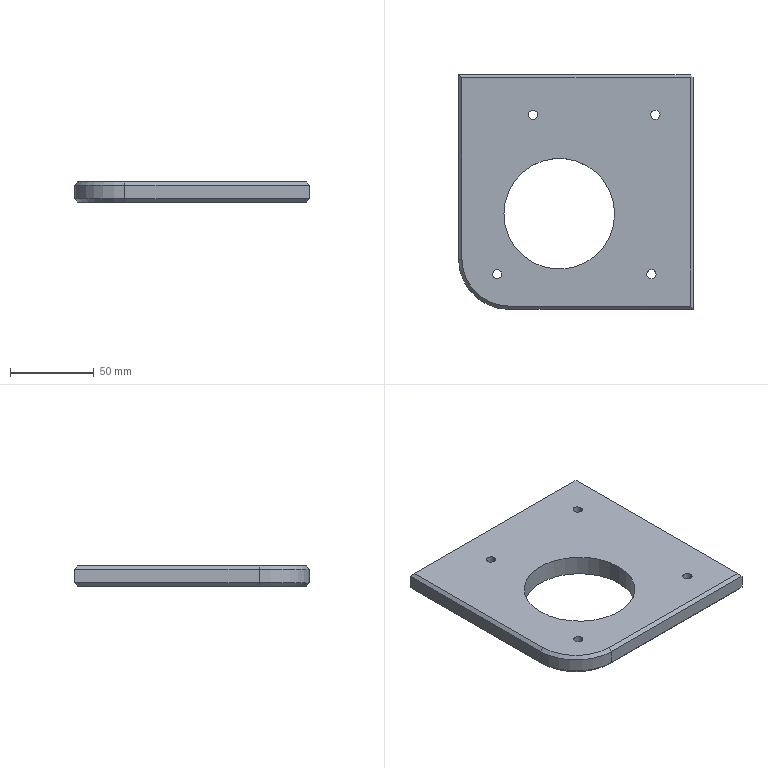Part | Creo | 1 solid | 40 faces | box 140 x 140 x 12 mm | volume 187371 mm3 | plane 19 | cylinder 19 | cone 2 | commonest cylinder face diameters 5.5 x8 9.5 x8 66 x2 60 x1
STEP:
#1=CARTESIAN_POINT('',(333.,236.995,1.));
#2=VERTEX_POINT('',#1);
#3=CARTESIAN_POINT('',(225.,236.995,1.));
#4=VERTEX_POINT('',#3);
#5=CARTESIAN_POINT('',(333.,236.995,1.));
#6=DIRECTION('',(-1.,0.,0.));
#7=VECTOR('',#6,108.);
#8=LINE('',#5,#7);
#9=EDGE_CURVE('',#2,#4,#8,.T.);
#10=ORIENTED_EDGE('',*,*,#9,.T.);
#11=CARTESIAN_POINT('',(197.,264.995,1.));
#12=VERTEX_POINT('',#11);
#13=CARTESIAN_POINT('',(225.,264.995,1.));
#14=DIRECTION('',(0.,0.,1.));
#15=DIRECTION('',(-1.,0.,0.));
#16=AXIS2_PLACEMENT_3D('',#13,#14,#15);
#17=CIRCLE('',#16,28.);
#18=EDGE_CURVE('',#12,#4,#17,.T.);
#19=ORIENTED_EDGE('',*,*,#18,.F.);
#20=CARTESIAN_POINT('',(197.,372.995,1.));
#21=VERTEX_POINT('',#20);
#22=CARTESIAN_POINT('',(197.,264.995,1.));
#23=DIRECTION('',(0.,1.,0.));
#24=VECTOR('',#23,108.);
#25=LINE('',#22,#24);
#26=EDGE_CURVE('',#12,#21,#25,.T.);
#27=ORIENTED_EDGE('',*,*,#26,.T.);
#28=CARTESIAN_POINT('',(333.,372.995,1.));
#29=VERTEX_POINT('',#28);
#30=CARTESIAN_POINT('',(197.,372.995,1.));
#31=DIRECTION('',(1.,0.,0.));
#32=VECTOR('',#31,136.);
#33=LINE('',#30,#32);
#34=EDGE_CURVE('',#21,#29,#33,.T.);
#35=ORIENTED_EDGE('',*,*,#34,.T.);
#36=CARTESIAN_POINT('',(333.,372.995,1.));
#37=DIRECTION('',(0.,-1.,0.));
#38=VECTOR('',#37,136.);
#39=LINE('',#36,#38);
#40=EDGE_CURVE('',#29,#2,#39,.T.);
#41=ORIENTED_EDGE('',*,*,#40,.T.);
#42=EDGE_LOOP('',(#10,#19,#27,#35,#41));
#43=FACE_OUTER_BOUND('',#42,.F.);
#44=CARTESIAN_POINT('',(215.25,256.,1.));
#45=VERTEX_POINT('',#44);
#46=CARTESIAN_POINT('',(220.75,256.,1.));
#47=VERTEX_POINT('',#46);
#48=CARTESIAN_POINT('',(218.,256.,1.));
#49=DIRECTION('',(0.,0.,-1.));
#50=DIRECTION('',(-1.,0.,0.));
#51=AXIS2_PLACEMENT_3D('',#48,#49,#50);
#52=CIRCLE('',#51,2.75);
#53=EDGE_CURVE('',#45,#47,#52,.T.);
#54=ORIENTED_EDGE('',*,*,#53,.F.);
#55=CARTESIAN_POINT('',(218.,256.,1.));
#56=DIRECTION('',(0.,0.,-1.));
#57=DIRECTION('',(1.,0.,0.));
#58=AXIS2_PLACEMENT_3D('',#55,#56,#57);
#59=CIRCLE('',#58,2.75);
#60=EDGE_CURVE('',#47,#45,#59,.T.);
#61=ORIENTED_EDGE('',*,*,#60,.F.);
#62=EDGE_LOOP('',(#54,#61));
#63=FACE_BOUND('',#62,.F.);
#64=CARTESIAN_POINT('',(236.618,351.,1.));
#65=VERTEX_POINT('',#64);
#66=CARTESIAN_POINT('',(242.118,351.,1.));
#67=VERTEX_POINT('',#66);
#68=CARTESIAN_POINT('',(239.368,351.,1.));
#69=DIRECTION('',(0.,0.,-1.));
#70=DIRECTION('',(-1.,0.,0.));
#71=AXIS2_PLACEMENT_3D('',#68,#69,#70);
#72=CIRCLE('',#71,2.75);
#73=EDGE_CURVE('',#65,#67,#72,.T.);
#74=ORIENTED_EDGE('',*,*,#73,.F.);
#75=CARTESIAN_POINT('',(239.368,351.,1.));
#76=DIRECTION('',(0.,0.,-1.));
#77=DIRECTION('',(1.,0.,0.));
#78=AXIS2_PLACEMENT_3D('',#75,#76,#77);
#79=CIRCLE('',#78,2.75);
#80=EDGE_CURVE('',#67,#65,#79,.T.);
#81=ORIENTED_EDGE('',*,*,#80,.F.);
#82=EDGE_LOOP('',(#74,#81));
#83=FACE_BOUND('',#82,.F.);
#84=CARTESIAN_POINT('',(288.,291.995,1.));
#85=VERTEX_POINT('',#84);
#86=CARTESIAN_POINT('',(222.,291.995,1.));
#87=VERTEX_POINT('',#86);
#88=CARTESIAN_POINT('',(255.,291.995,1.));
#89=DIRECTION('',(0.,0.,-1.));
#90=DIRECTION('',(1.,0.,0.));
#91=AXIS2_PLACEMENT_3D('',#88,#89,#90);
#92=CIRCLE('',#91,33.);
#93=EDGE_CURVE('',#85,#87,#92,.T.);
#94=ORIENTED_EDGE('',*,*,#93,.F.);
#95=CARTESIAN_POINT('',(255.,291.995,1.));
#96=DIRECTION('',(0.,0.,-1.));
#97=DIRECTION('',(-1.,0.,0.));
#98=AXIS2_PLACEMENT_3D('',#95,#96,#97);
#99=CIRCLE('',#98,33.);
#100=EDGE_CURVE('',#87,#85,#99,.T.);
#101=ORIENTED_EDGE('',*,*,#100,.F.);
#102=EDGE_LOOP('',(#94,#101));
#103=FACE_BOUND('',#102,.F.);
#104=CARTESIAN_POINT('',(309.618,351.,1.));
#105=VERTEX_POINT('',#104);
#106=CARTESIAN_POINT('',(315.118,351.,1.));
#107=VERTEX_POINT('',#106);
#108=CARTESIAN_POINT('',(312.368,351.,1.));
#109=DIRECTION('',(0.,0.,-1.));
#110=DIRECTION('',(-1.,0.,0.));
#111=AXIS2_PLACEMENT_3D('',#108,#109,#110);
#112=CIRCLE('',#111,2.75);
#113=EDGE_CURVE('',#105,#107,#112,.T.);
#114=ORIENTED_EDGE('',*,*,#113,.F.);
#115=CARTESIAN_POINT('',(312.368,351.,1.));
#116=DIRECTION('',(0.,0.,-1.));
#117=DIRECTION('',(1.,0.,0.));
#118=AXIS2_PLACEMENT_3D('',#115,#116,#117);
#119=CIRCLE('',#118,2.75);
#120=EDGE_CURVE('',#107,#105,#119,.T.);
#121=ORIENTED_EDGE('',*,*,#120,.F.);
#122=EDGE_LOOP('',(#114,#121));
#123=FACE_BOUND('',#122,.F.);
#124=CARTESIAN_POINT('',(307.25,256.,1.));
#125=VERTEX_POINT('',#124);
#126=CARTESIAN_POINT('',(312.75,256.,1.));
#127=VERTEX_POINT('',#126);
#128=CARTESIAN_POINT('',(310.,256.,1.));
#129=DIRECTION('',(0.,0.,-1.));
#130=DIRECTION('',(-1.,0.,0.));
#131=AXIS2_PLACEMENT_3D('',#128,#129,#130);
#132=CIRCLE('',#131,2.75);
#133=EDGE_CURVE('',#125,#127,#132,.T.);
#134=ORIENTED_EDGE('',*,*,#133,.F.);
#135=CARTESIAN_POINT('',(310.,256.,1.));
#136=DIRECTION('',(0.,0.,-1.));
#137=DIRECTION('',(1.,0.,0.));
#138=AXIS2_PLACEMENT_3D('',#135,#136,#137);
#139=CIRCLE('',#138,2.75);
#140=EDGE_CURVE('',#127,#125,#139,.T.);
#141=ORIENTED_EDGE('',*,*,#140,.F.);
#142=EDGE_LOOP('',(#134,#141));
#143=FACE_BOUND('',#142,.F.);
#144=CARTESIAN_POINT('',(265.,302.495,1.));
#145=DIRECTION('',(0.,0.,1.));
#146=DIRECTION('',(-1.,0.,0.));
#147=AXIS2_PLACEMENT_3D('',#144,#145,#146);
#148=PLANE('',#147);
#149=ADVANCED_FACE('',(#43,#63,#83,#103,#123,#143),#148,.T.);
#150=CARTESIAN_POINT('',(225.,234.995,-1.));
#151=VERTEX_POINT('',#150);
#152=CARTESIAN_POINT('',(335.,234.995,-1.));
#153=VERTEX_POINT('',#152);
#154=CARTESIAN_POINT('',(225.,234.995,-1.));
#155=DIRECTION('',(1.,0.,0.));
#156=VECTOR('',#155,110.);
#157=LINE('',#154,#156);
#158=EDGE_CURVE('',#151,#153,#157,.T.);
#159=ORIENTED_EDGE('',*,*,#158,.F.);
#160=CARTESIAN_POINT('',(225.,234.995,-1.));
#161=DIRECTION('',(0.,0.7071,0.7071));
#162=VECTOR('',#161,2.828);
#163=LINE('',#160,#162);
#164=EDGE_CURVE('',#151,#4,#163,.T.);
#165=ORIENTED_EDGE('',*,*,#164,.T.);
#166=ORIENTED_EDGE('',*,*,#9,.F.);
#167=CARTESIAN_POINT('',(333.,236.995,1.));
#168=DIRECTION('',(0.5774,-0.5774,-0.5774));
#169=VECTOR('',#168,3.464);
#170=LINE('',#167,#169);
#171=EDGE_CURVE('',#2,#153,#170,.T.);
#172=ORIENTED_EDGE('',*,*,#171,.T.);
#173=EDGE_LOOP('',(#159,#165,#166,#172));
#174=FACE_OUTER_BOUND('',#173,.F.);
#175=CARTESIAN_POINT('',(265.,234.995,-1.));
#176=DIRECTION('',(0.,0.7071,-0.7071));
#177=DIRECTION('',(-1.,0.,0.));
#178=AXIS2_PLACEMENT_3D('',#175,#176,#177);
#179=PLANE('',#178);
#180=ADVANCED_FACE('',(#174),#179,.F.);
#181=CARTESIAN_POINT('',(225.,234.995,-9.));
#182=VERTEX_POINT('',#181);
#183=CARTESIAN_POINT('',(225.,234.995,-9.));
#184=DIRECTION('',(0.,0.,1.));
#185=VECTOR('',#184,8.);
#186=LINE('',#183,#185);
#187=EDGE_CURVE('',#182,#151,#186,.T.);
#188=ORIENTED_EDGE('',*,*,#187,.T.);
#189=ORIENTED_EDGE('',*,*,#158,.T.);
#190=CARTESIAN_POINT('',(335.,234.995,-9.));
#191=VERTEX_POINT('',#190);
#192=CARTESIAN_POINT('',(335.,234.995,-1.));
#193=DIRECTION('',(0.,0.,-1.));
#194=VECTOR('',#193,8.);
#195=LINE('',#192,#194);
#196=EDGE_CURVE('',#153,#191,#195,.T.);
#197=ORIENTED_EDGE('',*,*,#196,.T.);
#198=CARTESIAN_POINT('',(335.,234.995,-9.));
#199=DIRECTION('',(-1.,0.,0.));
#200=VECTOR('',#199,110.);
#201=LINE('',#198,#200);
#202=EDGE_CURVE('',#191,#182,#201,.T.);
#203=ORIENTED_EDGE('',*,*,#202,.T.);
#204=EDGE_LOOP('',(#188,#189,#197,#203));
#205=FACE_OUTER_BOUND('',#204,.F.);
#206=CARTESIAN_POINT('',(265.,234.995,-11.));
#207=DIRECTION('',(0.,-1.,0.));
#208=DIRECTION('',(0.,0.,1.));
#209=AXIS2_PLACEMENT_3D('',#206,#207,#208);
#210=PLANE('',#209);
#211=ADVANCED_FACE('',(#205),#210,.T.);
#212=CARTESIAN_POINT('',(195.,264.995,-1.));
#213=VERTEX_POINT('',#212);
#214=CARTESIAN_POINT('',(195.,264.995,-9.));
#215=VERTEX_POINT('',#214);
#216=CARTESIAN_POINT('',(195.,264.995,-1.));
#217=DIRECTION('',(0.,0.,-1.));
#218=VECTOR('',#217,8.);
#219=LINE('',#216,#218);
#220=EDGE_CURVE('',#213,#215,#219,.T.);
#221=ORIENTED_EDGE('',*,*,#220,.F.);
#222=CARTESIAN_POINT('',(225.,264.995,-1.));
#223=DIRECTION('',(0.,0.,1.));
#224=DIRECTION('',(-1.,0.,0.));
#225=AXIS2_PLACEMENT_3D('',#222,#223,#224);
#226=CIRCLE('',#225,30.);
#227=EDGE_CURVE('',#213,#151,#226,.T.);
#228=ORIENTED_EDGE('',*,*,#227,.T.);
#229=ORIENTED_EDGE('',*,*,#187,.F.);
#230=CARTESIAN_POINT('',(225.,264.995,-9.));
#231=DIRECTION('',(0.,0.,-1.));
#232=DIRECTION('',(0.,-1.,0.));
#233=AXIS2_PLACEMENT_3D('',#230,#231,#232);
#234=CIRCLE('',#233,30.);
#235=EDGE_CURVE('',#182,#215,#234,.T.);
#236=ORIENTED_EDGE('',*,*,#235,.T.);
#237=EDGE_LOOP('',(#221,#228,#229,#236));
#238=FACE_OUTER_BOUND('',#237,.F.);
#239=CARTESIAN_POINT('',(225.,264.995,-11.));
#240=DIRECTION('',(0.,0.,1.));
#241=DIRECTION('',(-1.,0.,0.));
#242=AXIS2_PLACEMENT_3D('',#239,#240,#241);
#243=CYLINDRICAL_SURFACE('',#242,30.);
#244=ADVANCED_FACE('',(#238),#243,.T.);
#245=CARTESIAN_POINT('',(195.,374.995,-1.));
#246=VERTEX_POINT('',#245);
#247=CARTESIAN_POINT('',(195.,374.995,-9.));
#248=VERTEX_POINT('',#247);
#249=CARTESIAN_POINT('',(195.,374.995,-1.));
#250=DIRECTION('',(0.,0.,-1.));
#251=VECTOR('',#250,8.);
#252=LINE('',#249,#251);
#253=EDGE_CURVE('',#246,#248,#252,.T.);
#254=ORIENTED_EDGE('',*,*,#253,.F.);
#255=CARTESIAN_POINT('',(195.,374.995,-1.));
#256=DIRECTION('',(0.,-1.,0.));
#257=VECTOR('',#256,110.);
#258=LINE('',#255,#257);
#259=EDGE_CURVE('',#246,#213,#258,.T.);
#260=ORIENTED_EDGE('',*,*,#259,.T.);
#261=ORIENTED_EDGE('',*,*,#220,.T.);
#262=CARTESIAN_POINT('',(195.,264.995,-9.));
#263=DIRECTION('',(0.,1.,0.));
#264=VECTOR('',#263,110.);
#265=LINE('',#262,#264);
#266=EDGE_CURVE('',#215,#248,#265,.T.);
#267=ORIENTED_EDGE('',*,*,#266,.T.);
#268=EDGE_LOOP('',(#254,#260,#261,#267));
#269=FACE_OUTER_BOUND('',#268,.F.);
#270=CARTESIAN_POINT('',(195.,302.495,-11.));
#271=DIRECTION('',(-1.,0.,0.));
#272=DIRECTION('',(0.,0.,-1.));
#273=AXIS2_PLACEMENT_3D('',#270,#271,#272);
#274=PLANE('',#273);
#275=ADVANCED_FACE('',(#269),#274,.T.);
#276=ORIENTED_EDGE('',*,*,#253,.T.);
#277=CARTESIAN_POINT('',(333.,374.995,-9.));
#278=VERTEX_POINT('',#277);
#279=CARTESIAN_POINT('',(195.,374.995,-9.));
#280=DIRECTION('',(1.,0.,0.));
#281=VECTOR('',#280,138.);
#282=LINE('',#279,#281);
#283=EDGE_CURVE('',#248,#278,#282,.T.);
#284=ORIENTED_EDGE('',*,*,#283,.T.);
#285=CARTESIAN_POINT('',(333.,374.995,-1.));
#286=VERTEX_POINT('',#285);
#287=CARTESIAN_POINT('',(333.,374.995,-9.));
#288=DIRECTION('',(0.,0.,1.));
#289=VECTOR('',#288,8.);
#290=LINE('',#287,#289);
#291=EDGE_CURVE('',#278,#286,#290,.T.);
#292=ORIENTED_EDGE('',*,*,#291,.T.);
#293=CARTESIAN_POINT('',(333.,374.995,-1.));
#294=DIRECTION('',(-1.,0.,0.));
#295=VECTOR('',#294,138.);
#296=LINE('',#293,#295);
#297=EDGE_CURVE('',#286,#246,#296,.T.);
#298=ORIENTED_EDGE('',*,*,#297,.T.);
#299=EDGE_LOOP('',(#276,#284,#292,#298));
#300=FACE_OUTER_BOUND('',#299,.F.);
#301=CARTESIAN_POINT('',(285.,374.995,165.));
#302=DIRECTION('',(0.,1.,0.));
#303=DIRECTION('',(0.,0.,-1.));
#304=AXIS2_PLACEMENT_3D('',#301,#302,#303);
#305=PLANE('',#304);
#306=ADVANCED_FACE('',(#300),#305,.T.);
#307=CARTESIAN_POINT('',(333.,372.995,-11.));
#308=VERTEX_POINT('',#307);
#309=CARTESIAN_POINT('',(197.,372.995,-11.));
#310=VERTEX_POINT('',#309);
#311=CARTESIAN_POINT('',(333.,372.995,-11.));
#312=DIRECTION('',(-1.,0.,0.));
#313=VECTOR('',#312,136.);
#314=LINE('',#311,#313);
#315=EDGE_CURVE('',#308,#310,#314,.T.);
#316=ORIENTED_EDGE('',*,*,#315,.F.);
#317=CARTESIAN_POINT('',(334.,373.995,-10.));
#318=VERTEX_POINT('',#317);
#319=CARTESIAN_POINT('',(333.,372.995,-11.));
#320=DIRECTION('',(0.5774,0.5774,0.5774));
#321=VECTOR('',#320,1.732);
#322=LINE('',#319,#321);
#323=EDGE_CURVE('',#308,#318,#322,.T.);
#324=ORIENTED_EDGE('',*,*,#323,.T.);
#325=CARTESIAN_POINT('',(334.,373.995,-10.));
#326=DIRECTION('',(-0.5774,0.5774,0.5774));
#327=VECTOR('',#326,1.732);
#328=LINE('',#325,#327);
#329=EDGE_CURVE('',#318,#278,#328,.T.);
#330=ORIENTED_EDGE('',*,*,#329,.T.);
#331=ORIENTED_EDGE('',*,*,#283,.F.);
#332=CARTESIAN_POINT('',(195.,374.995,-9.));
#333=DIRECTION('',(0.5774,-0.5774,-0.5774));
#334=VECTOR('',#333,3.464);
#335=LINE('',#332,#334);
#336=EDGE_CURVE('',#248,#310,#335,.T.);
#337=ORIENTED_EDGE('',*,*,#336,.T.);
#338=EDGE_LOOP('',(#316,#324,#330,#331,#337));
#339=FACE_OUTER_BOUND('',#338,.F.);
#340=CARTESIAN_POINT('',(285.,374.995,-9.));
#341=DIRECTION('',(0.,-0.7071,0.7071));
#342=DIRECTION('',(-1.,0.,0.));
#343=AXIS2_PLACEMENT_3D('',#340,#341,#342);
#344=PLANE('',#343);
#345=ADVANCED_FACE('',(#339),#344,.F.);
#346=CARTESIAN_POINT('',(225.,236.995,-11.));
#347=VERTEX_POINT('',#346);
#348=CARTESIAN_POINT('',(197.,264.995,-11.));
#349=VERTEX_POINT('',#348);
#350=CARTESIAN_POINT('',(225.,264.995,-11.));
#351=DIRECTION('',(0.,0.,-1.));
#352=DIRECTION('',(0.,-1.,0.));
#353=AXIS2_PLACEMENT_3D('',#350,#351,#352);
#354=CIRCLE('',#353,28.);
#355=EDGE_CURVE('',#347,#349,#354,.T.);
#356=ORIENTED_EDGE('',*,*,#355,.F.);
#357=CARTESIAN_POINT('',(333.,236.995,-11.));
#358=VERTEX_POINT('',#357);
#359=CARTESIAN_POINT('',(225.,236.995,-11.));
#360=DIRECTION('',(1.,0.,0.));
#361=VECTOR('',#360,108.);
#362=LINE('',#359,#361);
#363=EDGE_CURVE('',#347,#358,#362,.T.);
#364=ORIENTED_EDGE('',*,*,#363,.T.);
#365=CARTESIAN_POINT('',(333.,236.995,-11.));
#366=DIRECTION('',(0.,1.,0.));
#367=VECTOR('',#366,136.);
#368=LINE('',#365,#367);
#369=EDGE_CURVE('',#358,#308,#368,.T.);
#370=ORIENTED_EDGE('',*,*,#369,.T.);
#371=ORIENTED_EDGE('',*,*,#315,.T.);
#372=CARTESIAN_POINT('',(197.,372.995,-11.));
#373=DIRECTION('',(0.,-1.,0.));
#374=VECTOR('',#373,108.);
#375=LINE('',#372,#374);
#376=EDGE_CURVE('',#310,#349,#375,.T.);
#377=ORIENTED_EDGE('',*,*,#376,.T.);
#378=EDGE_LOOP('',(#356,#364,#370,#371,#377));
#379=FACE_OUTER_BOUND('',#378,.F.);
#380=CARTESIAN_POINT('',(213.25,256.,-11.));
#381=VERTEX_POINT('',#380);
#382=CARTESIAN_POINT('',(222.75,256.,-11.));
#383=VERTEX_POINT('',#382);
#384=CARTESIAN_POINT('',(218.,256.,-11.));
#385=DIRECTION('',(0.,0.,1.));
#386=DIRECTION('',(-1.,0.,0.));
#387=AXIS2_PLACEMENT_3D('',#384,#385,#386);
#388=CIRCLE('',#387,4.75);
#389=EDGE_CURVE('',#381,#383,#388,.T.);
#390=ORIENTED_EDGE('',*,*,#389,.F.);
#391=CARTESIAN_POINT('',(218.,256.,-11.));
#392=DIRECTION('',(0.,0.,1.));
#393=DIRECTION('',(1.,0.,0.));
#394=AXIS2_PLACEMENT_3D('',#391,#392,#393);
#395=CIRCLE('',#394,4.75);
#396=EDGE_CURVE('',#383,#381,#395,.T.);
#397=ORIENTED_EDGE('',*,*,#396,.F.);
#398=EDGE_LOOP('',(#390,#397));
#399=FACE_BOUND('',#398,.F.);
#400=CARTESIAN_POINT('',(307.618,351.,-11.));
#401=VERTEX_POINT('',#400);
#402=CARTESIAN_POINT('',(317.118,351.,-11.));
#403=VERTEX_POINT('',#402);
#404=CARTESIAN_POINT('',(312.368,351.,-11.));
#405=DIRECTION('',(0.,0.,1.));
#406=DIRECTION('',(-1.,0.,0.));
#407=AXIS2_PLACEMENT_3D('',#404,#405,#406);
#408=CIRCLE('',#407,4.75);
#409=EDGE_CURVE('',#401,#403,#408,.T.);
#410=ORIENTED_EDGE('',*,*,#409,.F.);
#411=CARTESIAN_POINT('',(312.368,351.,-11.));
#412=DIRECTION('',(0.,0.,1.));
#413=DIRECTION('',(1.,0.,0.));
#414=AXIS2_PLACEMENT_3D('',#411,#412,#413);
#415=CIRCLE('',#414,4.75);
#416=EDGE_CURVE('',#403,#401,#415,.T.);
#417=ORIENTED_EDGE('',*,*,#416,.F.);
#418=EDGE_LOOP('',(#410,#417));
#419=FACE_BOUND('',#418,.F.);
#420=CARTESIAN_POINT('',(234.618,351.,-11.));
#421=VERTEX_POINT('',#420);
#422=CARTESIAN_POINT('',(244.118,351.,-11.));
#423=VERTEX_POINT('',#422);
#424=CARTESIAN_POINT('',(239.368,351.,-11.));
#425=DIRECTION('',(0.,0.,1.));
#426=DIRECTION('',(-1.,0.,0.));
#427=AXIS2_PLACEMENT_3D('',#424,#425,#426);
#428=CIRCLE('',#427,4.75);
#429=EDGE_CURVE('',#421,#423,#428,.T.);
#430=ORIENTED_EDGE('',*,*,#429,.F.);
#431=CARTESIAN_POINT('',(239.368,351.,-11.));
#432=DIRECTION('',(0.,0.,1.));
#433=DIRECTION('',(1.,0.,0.));
#434=AXIS2_PLACEMENT_3D('',#431,#432,#433);
#435=CIRCLE('',#434,4.75);
#436=EDGE_CURVE('',#423,#421,#435,.T.);
#437=ORIENTED_EDGE('',*,*,#436,.F.);
#438=EDGE_LOOP('',(#430,#437));
#439=FACE_BOUND('',#438,.F.);
#440=CARTESIAN_POINT('',(305.25,256.,-11.));
#441=VERTEX_POINT('',#440);
#442=CARTESIAN_POINT('',(314.75,256.,-11.));
#443=VERTEX_POINT('',#442);
#444=CARTESIAN_POINT('',(310.,256.,-11.));
#445=DIRECTION('',(0.,0.,1.));
#446=DIRECTION('',(-1.,0.,0.));
#447=AXIS2_PLACEMENT_3D('',#444,#445,#446);
#448=CIRCLE('',#447,4.75);
#449=EDGE_CURVE('',#441,#443,#448,.T.);
#450=ORIENTED_EDGE('',*,*,#449,.F.);
#451=CARTESIAN_POINT('',(310.,256.,-11.));
#452=DIRECTION('',(0.,0.,1.));
#453=DIRECTION('',(1.,0.,0.));
#454=AXIS2_PLACEMENT_3D('',#451,#452,#453);
#455=CIRCLE('',#454,4.75);
#456=EDGE_CURVE('',#443,#441,#455,.T.);
#457=ORIENTED_EDGE('',*,*,#456,.F.);
#458=EDGE_LOOP('',(#450,#457));
#459=FACE_BOUND('',#458,.F.);
#460=CARTESIAN_POINT('',(222.,291.995,-11.));
#461=VERTEX_POINT('',#460);
#462=CARTESIAN_POINT('',(288.,291.995,-11.));
#463=VERTEX_POINT('',#462);
#464=CARTESIAN_POINT('',(255.,291.995,-11.));
#465=DIRECTION('',(0.,0.,1.));
#466=DIRECTION('',(-1.,0.,0.));
#467=AXIS2_PLACEMENT_3D('',#464,#465,#466);
#468=CIRCLE('',#467,33.);
#469=EDGE_CURVE('',#461,#463,#468,.T.);
#470=ORIENTED_EDGE('',*,*,#469,.F.);
#471=CARTESIAN_POINT('',(255.,291.995,-11.));
#472=DIRECTION('',(0.,0.,1.));
#473=DIRECTION('',(1.,0.,0.));
#474=AXIS2_PLACEMENT_3D('',#471,#472,#473);
#475=CIRCLE('',#474,33.);
#476=EDGE_CURVE('',#463,#461,#475,.T.);
#477=ORIENTED_EDGE('',*,*,#476,.F.);
#478=EDGE_LOOP('',(#470,#477));
#479=FACE_BOUND('',#478,.F.);
#480=CARTESIAN_POINT('',(265.,302.495,-11.));
#481=DIRECTION('',(0.,0.,-1.));
#482=DIRECTION('',(1.,0.,0.));
#483=AXIS2_PLACEMENT_3D('',#480,#481,#482);
#484=PLANE('',#483);
#485=ADVANCED_FACE('',(#379,#399,#419,#439,#459,#479),#484,.T.);
#486=CARTESIAN_POINT('',(314.75,256.,-5.));
#487=VERTEX_POINT('',#486);
#488=CARTESIAN_POINT('',(305.25,256.,-5.));
#489=VERTEX_POINT('',#488);
#490=CARTESIAN_POINT('',(310.,256.,-5.));
#491=DIRECTION('',(0.,0.,-1.));
#492=DIRECTION('',(1.,0.,0.));
#493=AXIS2_PLACEMENT_3D('',#490,#491,#492);
#494=CIRCLE('',#493,4.75);
#495=EDGE_CURVE('',#487,#489,#494,.T.);
#496=ORIENTED_EDGE('',*,*,#495,.T.);
#497=CARTESIAN_POINT('',(305.25,256.,-5.));
#498=DIRECTION('',(0.,0.,-1.));
#499=VECTOR('',#498,6.);
#500=LINE('',#497,#499);
#501=EDGE_CURVE('',#489,#441,#500,.T.);
#502=ORIENTED_EDGE('',*,*,#501,.T.);
#503=ORIENTED_EDGE('',*,*,#449,.T.);
#504=CARTESIAN_POINT('',(314.75,256.,-5.));
#505=DIRECTION('',(0.,0.,-1.));
#506=VECTOR('',#505,6.);
#507=LINE('',#504,#506);
#508=EDGE_CURVE('',#487,#443,#507,.T.);
#509=ORIENTED_EDGE('',*,*,#508,.F.);
#510=EDGE_LOOP('',(#496,#502,#503,#509));
#511=FACE_OUTER_BOUND('',#510,.F.);
#512=CARTESIAN_POINT('',(310.,256.,-11.));
#513=DIRECTION('',(0.,0.,-1.));
#514=DIRECTION('',(-1.,0.,0.));
#515=AXIS2_PLACEMENT_3D('',#512,#513,#514);
#516=CYLINDRICAL_SURFACE('',#515,4.75);
#517=ADVANCED_FACE('',(#511),#516,.F.);
#518=CARTESIAN_POINT('',(310.,256.,-5.));
#519=DIRECTION('',(0.,0.,-1.));
#520=DIRECTION('',(-1.,0.,0.));
#521=AXIS2_PLACEMENT_3D('',#518,#519,#520);
#522=CIRCLE('',#521,4.75);
#523=EDGE_CURVE('',#489,#487,#522,.T.);
#524=ORIENTED_EDGE('',*,*,#523,.F.);
#525=ORIENTED_EDGE('',*,*,#495,.F.);
#526=EDGE_LOOP('',(#524,#525));
#527=FACE_OUTER_BOUND('',#526,.F.);
#528=CARTESIAN_POINT('',(307.25,256.,-5.));
#529=VERTEX_POINT('',#528);
#530=CARTESIAN_POINT('',(312.75,256.,-5.));
#531=VERTEX_POINT('',#530);
#532=CARTESIAN_POINT('',(310.,256.,-5.));
#533=DIRECTION('',(0.,0.,1.));
#534=DIRECTION('',(-1.,0.,0.));
#535=AXIS2_PLACEMENT_3D('',#532,#533,#534);
#536=CIRCLE('',#535,2.75);
#537=EDGE_CURVE('',#529,#531,#536,.T.);
#538=ORIENTED_EDGE('',*,*,#537,.F.);
#539=CARTESIAN_POINT('',(310.,256.,-5.));
#540=DIRECTION('',(0.,0.,1.));
#541=DIRECTION('',(1.,0.,0.));
#542=AXIS2_PLACEMENT_3D('',#539,#540,#541);
#543=CIRCLE('',#542,2.75);
#544=EDGE_CURVE('',#531,#529,#543,.T.);
#545=ORIENTED_EDGE('',*,*,#544,.F.);
#546=EDGE_LOOP('',(#538,#545));
#547=FACE_BOUND('',#546,.F.);
#548=CARTESIAN_POINT('',(310.,260.75,-5.));
#549=DIRECTION('',(0.,0.,1.));
#550=DIRECTION('',(1.,0.,0.));
#551=AXIS2_PLACEMENT_3D('',#548,#549,#550);
#552=PLANE('',#551);
#553=ADVANCED_FACE('',(#527,#547),#552,.F.);
#554=ORIENTED_EDGE('',*,*,#140,.T.);
#555=CARTESIAN_POINT('',(307.25,256.,1.));
#556=DIRECTION('',(0.,0.,-1.));
#557=VECTOR('',#556,6.);
#558=LINE('',#555,#557);
#559=EDGE_CURVE('',#125,#529,#558,.T.);
#560=ORIENTED_EDGE('',*,*,#559,.T.);
#561=ORIENTED_EDGE('',*,*,#537,.T.);
#562=CARTESIAN_POINT('',(312.75,256.,1.));
#563=DIRECTION('',(0.,0.,-1.));
#564=VECTOR('',#563,6.);
#565=LINE('',#562,#564);
#566=EDGE_CURVE('',#127,#531,#565,.T.);
#567=ORIENTED_EDGE('',*,*,#566,.F.);
#568=EDGE_LOOP('',(#554,#560,#561,#567));
#569=FACE_OUTER_BOUND('',#568,.F.);
#570=CARTESIAN_POINT('',(310.,256.,-11.));
#571=DIRECTION('',(0.,0.,-1.));
#572=DIRECTION('',(-1.,0.,0.));
#573=AXIS2_PLACEMENT_3D('',#570,#571,#572);
#574=CYLINDRICAL_SURFACE('',#573,2.75);
#575=ADVANCED_FACE('',(#569),#574,.F.);
#576=ORIENTED_EDGE('',*,*,#133,.T.);
#577=ORIENTED_EDGE('',*,*,#566,.T.);
#578=ORIENTED_EDGE('',*,*,#544,.T.);
#579=ORIENTED_EDGE('',*,*,#559,.F.);
#580=EDGE_LOOP('',(#576,#577,#578,#579));
#581=FACE_OUTER_BOUND('',#580,.F.);
#582=CARTESIAN_POINT('',(310.,256.,-11.));
#583=DIRECTION('',(0.,0.,-1.));
#584=DIRECTION('',(-1.,0.,0.));
#585=AXIS2_PLACEMENT_3D('',#582,#583,#584);
#586=CYLINDRICAL_SURFACE('',#585,2.75);
#587=ADVANCED_FACE('',(#581),#586,.F.);
#588=ORIENTED_EDGE('',*,*,#523,.T.);
#589=ORIENTED_EDGE('',*,*,#508,.T.);
#590=ORIENTED_EDGE('',*,*,#456,.T.);
#591=ORIENTED_EDGE('',*,*,#501,.F.);
#592=EDGE_LOOP('',(#588,#589,#590,#591));
#593=FACE_OUTER_BOUND('',#592,.F.);
#594=CARTESIAN_POINT('',(310.,256.,-11.));
#595=DIRECTION('',(0.,0.,-1.));
#596=DIRECTION('',(-1.,0.,0.));
#597=AXIS2_PLACEMENT_3D('',#594,#595,#596);
#598=CYLINDRICAL_SURFACE('',#597,4.75);
#599=ADVANCED_FACE('',(#593),#598,.F.);
#600=CARTESIAN_POINT('',(222.75,256.,-5.));
#601=VERTEX_POINT('',#600);
#602=CARTESIAN_POINT('',(213.25,256.,-5.));
#603=VERTEX_POINT('',#602);
#604=CARTESIAN_POINT('',(218.,256.,-5.));
#605=DIRECTION('',(0.,0.,-1.));
#606=DIRECTION('',(1.,0.,0.));
#607=AXIS2_PLACEMENT_3D('',#604,#605,#606);
#608=CIRCLE('',#607,4.75);
#609=EDGE_CURVE('',#601,#603,#608,.T.);
#610=ORIENTED_EDGE('',*,*,#609,.T.);
#611=CARTESIAN_POINT('',(213.25,256.,-5.));
#612=DIRECTION('',(0.,0.,-1.));
#613=VECTOR('',#612,6.);
#614=LINE('',#611,#613);
#615=EDGE_CURVE('',#603,#381,#614,.T.);
#616=ORIENTED_EDGE('',*,*,#615,.T.);
#617=ORIENTED_EDGE('',*,*,#389,.T.);
#618=CARTESIAN_POINT('',(222.75,256.,-5.));
#619=DIRECTION('',(0.,0.,-1.));
#620=VECTOR('',#619,6.);
#621=LINE('',#618,#620);
#622=EDGE_CURVE('',#601,#383,#621,.T.);
#623=ORIENTED_EDGE('',*,*,#622,.F.);
#624=EDGE_LOOP('',(#610,#616,#617,#623));
#625=FACE_OUTER_BOUND('',#624,.F.);
#626=CARTESIAN_POINT('',(218.,256.,-11.));
#627=DIRECTION('',(0.,0.,-1.));
#628=DIRECTION('',(-1.,0.,0.));
#629=AXIS2_PLACEMENT_3D('',#626,#627,#628);
#630=CYLINDRICAL_SURFACE('',#629,4.75);
#631=ADVANCED_FACE('',(#625),#630,.F.);
#632=CARTESIAN_POINT('',(218.,256.,-5.));
#633=DIRECTION('',(0.,0.,-1.));
#634=DIRECTION('',(-1.,0.,0.));
#635=AXIS2_PLACEMENT_3D('',#632,#633,#634);
#636=CIRCLE('',#635,4.75);
#637=EDGE_CURVE('',#603,#601,#636,.T.);
#638=ORIENTED_EDGE('',*,*,#637,.F.);
#639=ORIENTED_EDGE('',*,*,#609,.F.);
#640=EDGE_LOOP('',(#638,#639));
#641=FACE_OUTER_BOUND('',#640,.F.);
#642=CARTESIAN_POINT('',(215.25,256.,-5.));
#643=VERTEX_POINT('',#642);
#644=CARTESIAN_POINT('',(220.75,256.,-5.));
#645=VERTEX_POINT('',#644);
#646=CARTESIAN_POINT('',(218.,256.,-5.));
#647=DIRECTION('',(0.,0.,1.));
#648=DIRECTION('',(-1.,0.,0.));
#649=AXIS2_PLACEMENT_3D('',#646,#647,#648);
#650=CIRCLE('',#649,2.75);
#651=EDGE_CURVE('',#643,#645,#650,.T.);
#652=ORIENTED_EDGE('',*,*,#651,.F.);
#653=CARTESIAN_POINT('',(218.,256.,-5.));
#654=DIRECTION('',(0.,0.,1.));
#655=DIRECTION('',(1.,0.,0.));
#656=AXIS2_PLACEMENT_3D('',#653,#654,#655);
#657=CIRCLE('',#656,2.75);
#658=EDGE_CURVE('',#645,#643,#657,.T.);
#659=ORIENTED_EDGE('',*,*,#658,.F.);
#660=EDGE_LOOP('',(#652,#659));
#661=FACE_BOUND('',#660,.F.);
#662=CARTESIAN_POINT('',(218.,260.75,-5.));
#663=DIRECTION('',(0.,0.,1.));
#664=DIRECTION('',(1.,0.,0.));
#665=AXIS2_PLACEMENT_3D('',#662,#663,#664);
#666=PLANE('',#665);
#667=ADVANCED_FACE('',(#641,#661),#666,.F.);
#668=ORIENTED_EDGE('',*,*,#60,.T.);
#669=CARTESIAN_POINT('',(215.25,256.,1.));
#670=DIRECTION('',(0.,0.,-1.));
#671=VECTOR('',#670,6.);
#672=LINE('',#669,#671);
#673=EDGE_CURVE('',#45,#643,#672,.T.);
#674=ORIENTED_EDGE('',*,*,#673,.T.);
#675=ORIENTED_EDGE('',*,*,#651,.T.);
#676=CARTESIAN_POINT('',(220.75,256.,1.));
#677=DIRECTION('',(0.,0.,-1.));
#678=VECTOR('',#677,6.);
#679=LINE('',#676,#678);
#680=EDGE_CURVE('',#47,#645,#679,.T.);
#681=ORIENTED_EDGE('',*,*,#680,.F.);
#682=EDGE_LOOP('',(#668,#674,#675,#681));
#683=FACE_OUTER_BOUND('',#682,.F.);
#684=CARTESIAN_POINT('',(218.,256.,-11.));
#685=DIRECTION('',(0.,0.,-1.));
#686=DIRECTION('',(-1.,0.,0.));
#687=AXIS2_PLACEMENT_3D('',#684,#685,#686);
#688=CYLINDRICAL_SURFACE('',#687,2.75);
#689=ADVANCED_FACE('',(#683),#688,.F.);
#690=ORIENTED_EDGE('',*,*,#53,.T.);
#691=ORIENTED_EDGE('',*,*,#680,.T.);
#692=ORIENTED_EDGE('',*,*,#658,.T.);
#693=ORIENTED_EDGE('',*,*,#673,.F.);
#694=EDGE_LOOP('',(#690,#691,#692,#693));
#695=FACE_OUTER_BOUND('',#694,.F.);
#696=CARTESIAN_POINT('',(218.,256.,-11.));
#697=DIRECTION('',(0.,0.,-1.));
#698=DIRECTION('',(-1.,0.,0.));
#699=AXIS2_PLACEMENT_3D('',#696,#697,#698);
#700=CYLINDRICAL_SURFACE('',#699,2.75);
#701=ADVANCED_FACE('',(#695),#700,.F.);
#702=ORIENTED_EDGE('',*,*,#637,.T.);
#703=ORIENTED_EDGE('',*,*,#622,.T.);
#704=ORIENTED_EDGE('',*,*,#396,.T.);
#705=ORIENTED_EDGE('',*,*,#615,.F.);
#706=EDGE_LOOP('',(#702,#703,#704,#705));
#707=FACE_OUTER_BOUND('',#706,.F.);
#708=CARTESIAN_POINT('',(218.,256.,-11.));
#709=DIRECTION('',(0.,0.,-1.));
#710=DIRECTION('',(-1.,0.,0.));
#711=AXIS2_PLACEMENT_3D('',#708,#709,#710);
#712=CYLINDRICAL_SURFACE('',#711,4.75);
#713=ADVANCED_FACE('',(#707),#712,.F.);
#714=CARTESIAN_POINT('',(317.118,351.,-5.));
#715=VERTEX_POINT('',#714);
#716=CARTESIAN_POINT('',(307.618,351.,-5.));
#717=VERTEX_POINT('',#716);
#718=CARTESIAN_POINT('',(312.368,351.,-5.));
#719=DIRECTION('',(0.,0.,-1.));
#720=DIRECTION('',(1.,0.,0.));
#721=AXIS2_PLACEMENT_3D('',#718,#719,#720);
#722=CIRCLE('',#721,4.75);
#723=EDGE_CURVE('',#715,#717,#722,.T.);
#724=ORIENTED_EDGE('',*,*,#723,.T.);
#725=CARTESIAN_POINT('',(307.618,351.,-5.));
#726=DIRECTION('',(0.,0.,-1.));
#727=VECTOR('',#726,6.);
#728=LINE('',#725,#727);
#729=EDGE_CURVE('',#717,#401,#728,.T.);
#730=ORIENTED_EDGE('',*,*,#729,.T.);
#731=ORIENTED_EDGE('',*,*,#409,.T.);
#732=CARTESIAN_POINT('',(317.118,351.,-5.));
#733=DIRECTION('',(0.,0.,-1.));
#734=VECTOR('',#733,6.);
#735=LINE('',#732,#734);
#736=EDGE_CURVE('',#715,#403,#735,.T.);
#737=ORIENTED_EDGE('',*,*,#736,.F.);
#738=EDGE_LOOP('',(#724,#730,#731,#737));
#739=FACE_OUTER_BOUND('',#738,.F.);
#740=CARTESIAN_POINT('',(312.368,351.,-11.));
#741=DIRECTION('',(0.,0.,-1.));
#742=DIRECTION('',(-1.,0.,0.));
#743=AXIS2_PLACEMENT_3D('',#740,#741,#742);
#744=CYLINDRICAL_SURFACE('',#743,4.75);
#745=ADVANCED_FACE('',(#739),#744,.F.);
#746=CARTESIAN_POINT('',(312.368,351.,-5.));
#747=DIRECTION('',(0.,0.,-1.));
#748=DIRECTION('',(-1.,0.,0.));
#749=AXIS2_PLACEMENT_3D('',#746,#747,#748);
#750=CIRCLE('',#749,4.75);
#751=EDGE_CURVE('',#717,#715,#750,.T.);
#752=ORIENTED_EDGE('',*,*,#751,.F.);
#753=ORIENTED_EDGE('',*,*,#723,.F.);
#754=EDGE_LOOP('',(#752,#753));
#755=FACE_OUTER_BOUND('',#754,.F.);
#756=CARTESIAN_POINT('',(309.618,351.,-5.));
#757=VERTEX_POINT('',#756);
#758=CARTESIAN_POINT('',(315.118,351.,-5.));
#759=VERTEX_POINT('',#758);
#760=CARTESIAN_POINT('',(312.368,351.,-5.));
#761=DIRECTION('',(0.,0.,1.));
#762=DIRECTION('',(-1.,0.,0.));
#763=AXIS2_PLACEMENT_3D('',#760,#761,#762);
#764=CIRCLE('',#763,2.75);
#765=EDGE_CURVE('',#757,#759,#764,.T.);
#766=ORIENTED_EDGE('',*,*,#765,.F.);
#767=CARTESIAN_POINT('',(312.368,351.,-5.));
#768=DIRECTION('',(0.,0.,1.));
#769=DIRECTION('',(1.,0.,0.));
#770=AXIS2_PLACEMENT_3D('',#767,#768,#769);
#771=CIRCLE('',#770,2.75);
#772=EDGE_CURVE('',#759,#757,#771,.T.);
#773=ORIENTED_EDGE('',*,*,#772,.F.);
#774=EDGE_LOOP('',(#766,#773));
#775=FACE_BOUND('',#774,.F.);
#776=CARTESIAN_POINT('',(312.368,355.75,-5.));
#777=DIRECTION('',(0.,0.,1.));
#778=DIRECTION('',(1.,0.,0.));
#779=AXIS2_PLACEMENT_3D('',#776,#777,#778);
#780=PLANE('',#779);
#781=ADVANCED_FACE('',(#755,#775),#780,.F.);
#782=ORIENTED_EDGE('',*,*,#120,.T.);
#783=CARTESIAN_POINT('',(309.618,351.,1.));
#784=DIRECTION('',(0.,0.,-1.));
#785=VECTOR('',#784,6.);
#786=LINE('',#783,#785);
#787=EDGE_CURVE('',#105,#757,#786,.T.);
#788=ORIENTED_EDGE('',*,*,#787,.T.);
#789=ORIENTED_EDGE('',*,*,#765,.T.);
#790=CARTESIAN_POINT('',(315.118,351.,1.));
#791=DIRECTION('',(0.,0.,-1.));
#792=VECTOR('',#791,6.);
#793=LINE('',#790,#792);
#794=EDGE_CURVE('',#107,#759,#793,.T.);
#795=ORIENTED_EDGE('',*,*,#794,.F.);
#796=EDGE_LOOP('',(#782,#788,#789,#795));
#797=FACE_OUTER_BOUND('',#796,.F.);
#798=CARTESIAN_POINT('',(312.368,351.,-11.));
#799=DIRECTION('',(0.,0.,-1.));
#800=DIRECTION('',(-1.,0.,0.));
#801=AXIS2_PLACEMENT_3D('',#798,#799,#800);
#802=CYLINDRICAL_SURFACE('',#801,2.75);
#803=ADVANCED_FACE('',(#797),#802,.F.);
#804=ORIENTED_EDGE('',*,*,#113,.T.);
#805=ORIENTED_EDGE('',*,*,#794,.T.);
#806=ORIENTED_EDGE('',*,*,#772,.T.);
#807=ORIENTED_EDGE('',*,*,#787,.F.);
#808=EDGE_LOOP('',(#804,#805,#806,#807));
#809=FACE_OUTER_BOUND('',#808,.F.);
#810=CARTESIAN_POINT('',(312.368,351.,-11.));
#811=DIRECTION('',(0.,0.,-1.));
#812=DIRECTION('',(-1.,0.,0.));
#813=AXIS2_PLACEMENT_3D('',#810,#811,#812);
#814=CYLINDRICAL_SURFACE('',#813,2.75);
#815=ADVANCED_FACE('',(#809),#814,.F.);
#816=ORIENTED_EDGE('',*,*,#751,.T.);
#817=ORIENTED_EDGE('',*,*,#736,.T.);
#818=ORIENTED_EDGE('',*,*,#416,.T.);
#819=ORIENTED_EDGE('',*,*,#729,.F.);
#820=EDGE_LOOP('',(#816,#817,#818,#819));
#821=FACE_OUTER_BOUND('',#820,.F.);
#822=CARTESIAN_POINT('',(312.368,351.,-11.));
#823=DIRECTION('',(0.,0.,-1.));
#824=DIRECTION('',(-1.,0.,0.));
#825=AXIS2_PLACEMENT_3D('',#822,#823,#824);
#826=CYLINDRICAL_SURFACE('',#825,4.75);
#827=ADVANCED_FACE('',(#821),#826,.F.);
#828=CARTESIAN_POINT('',(244.118,351.,-5.));
#829=VERTEX_POINT('',#828);
#830=CARTESIAN_POINT('',(234.618,351.,-5.));
#831=VERTEX_POINT('',#830);
#832=CARTESIAN_POINT('',(239.368,351.,-5.));
#833=DIRECTION('',(0.,0.,-1.));
#834=DIRECTION('',(1.,0.,0.));
#835=AXIS2_PLACEMENT_3D('',#832,#833,#834);
#836=CIRCLE('',#835,4.75);
#837=EDGE_CURVE('',#829,#831,#836,.T.);
#838=ORIENTED_EDGE('',*,*,#837,.T.);
#839=CARTESIAN_POINT('',(234.618,351.,-5.));
#840=DIRECTION('',(0.,0.,-1.));
#841=VECTOR('',#840,6.);
#842=LINE('',#839,#841);
#843=EDGE_CURVE('',#831,#421,#842,.T.);
#844=ORIENTED_EDGE('',*,*,#843,.T.);
#845=ORIENTED_EDGE('',*,*,#429,.T.);
#846=CARTESIAN_POINT('',(244.118,351.,-5.));
#847=DIRECTION('',(0.,0.,-1.));
#848=VECTOR('',#847,6.);
#849=LINE('',#846,#848);
#850=EDGE_CURVE('',#829,#423,#849,.T.);
#851=ORIENTED_EDGE('',*,*,#850,.F.);
#852=EDGE_LOOP('',(#838,#844,#845,#851));
#853=FACE_OUTER_BOUND('',#852,.F.);
#854=CARTESIAN_POINT('',(239.368,351.,-11.));
#855=DIRECTION('',(0.,0.,-1.));
#856=DIRECTION('',(-1.,0.,0.));
#857=AXIS2_PLACEMENT_3D('',#854,#855,#856);
#858=CYLINDRICAL_SURFACE('',#857,4.75);
#859=ADVANCED_FACE('',(#853),#858,.F.);
#860=CARTESIAN_POINT('',(239.368,351.,-5.));
#861=DIRECTION('',(0.,0.,-1.));
#862=DIRECTION('',(-1.,0.,0.));
#863=AXIS2_PLACEMENT_3D('',#860,#861,#862);
#864=CIRCLE('',#863,4.75);
#865=EDGE_CURVE('',#831,#829,#864,.T.);
#866=ORIENTED_EDGE('',*,*,#865,.F.);
#867=ORIENTED_EDGE('',*,*,#837,.F.);
#868=EDGE_LOOP('',(#866,#867));
#869=FACE_OUTER_BOUND('',#868,.F.);
#870=CARTESIAN_POINT('',(236.618,351.,-5.));
#871=VERTEX_POINT('',#870);
#872=CARTESIAN_POINT('',(242.118,351.,-5.));
#873=VERTEX_POINT('',#872);
#874=CARTESIAN_POINT('',(239.368,351.,-5.));
#875=DIRECTION('',(0.,0.,1.));
#876=DIRECTION('',(-1.,0.,0.));
#877=AXIS2_PLACEMENT_3D('',#874,#875,#876);
#878=CIRCLE('',#877,2.75);
#879=EDGE_CURVE('',#871,#873,#878,.T.);
#880=ORIENTED_EDGE('',*,*,#879,.F.);
#881=CARTESIAN_POINT('',(239.368,351.,-5.));
#882=DIRECTION('',(0.,0.,1.));
#883=DIRECTION('',(1.,0.,0.));
#884=AXIS2_PLACEMENT_3D('',#881,#882,#883);
#885=CIRCLE('',#884,2.75);
#886=EDGE_CURVE('',#873,#871,#885,.T.);
#887=ORIENTED_EDGE('',*,*,#886,.F.);
#888=EDGE_LOOP('',(#880,#887));
#889=FACE_BOUND('',#888,.F.);
#890=CARTESIAN_POINT('',(239.368,355.75,-5.));
#891=DIRECTION('',(0.,0.,1.));
#892=DIRECTION('',(1.,0.,0.));
#893=AXIS2_PLACEMENT_3D('',#890,#891,#892);
#894=PLANE('',#893);
#895=ADVANCED_FACE('',(#869,#889),#894,.F.);
#896=ORIENTED_EDGE('',*,*,#80,.T.);
#897=CARTESIAN_POINT('',(236.618,351.,1.));
#898=DIRECTION('',(0.,0.,-1.));
#899=VECTOR('',#898,6.);
#900=LINE('',#897,#899);
#901=EDGE_CURVE('',#65,#871,#900,.T.);
#902=ORIENTED_EDGE('',*,*,#901,.T.);
#903=ORIENTED_EDGE('',*,*,#879,.T.);
#904=CARTESIAN_POINT('',(242.118,351.,1.));
#905=DIRECTION('',(0.,0.,-1.));
#906=VECTOR('',#905,6.);
#907=LINE('',#904,#906);
#908=EDGE_CURVE('',#67,#873,#907,.T.);
#909=ORIENTED_EDGE('',*,*,#908,.F.);
#910=EDGE_LOOP('',(#896,#902,#903,#909));
#911=FACE_OUTER_BOUND('',#910,.F.);
#912=CARTESIAN_POINT('',(239.368,351.,-11.));
#913=DIRECTION('',(0.,0.,-1.));
#914=DIRECTION('',(-1.,0.,0.));
#915=AXIS2_PLACEMENT_3D('',#912,#913,#914);
#916=CYLINDRICAL_SURFACE('',#915,2.75);
#917=ADVANCED_FACE('',(#911),#916,.F.);
#918=ORIENTED_EDGE('',*,*,#73,.T.);
#919=ORIENTED_EDGE('',*,*,#908,.T.);
#920=ORIENTED_EDGE('',*,*,#886,.T.);
#921=ORIENTED_EDGE('',*,*,#901,.F.);
#922=EDGE_LOOP('',(#918,#919,#920,#921));
#923=FACE_OUTER_BOUND('',#922,.F.);
#924=CARTESIAN_POINT('',(239.368,351.,-11.));
#925=DIRECTION('',(0.,0.,-1.));
#926=DIRECTION('',(-1.,0.,0.));
#927=AXIS2_PLACEMENT_3D('',#924,#925,#926);
#928=CYLINDRICAL_SURFACE('',#927,2.75);
#929=ADVANCED_FACE('',(#923),#928,.F.);
#930=ORIENTED_EDGE('',*,*,#865,.T.);
#931=ORIENTED_EDGE('',*,*,#850,.T.);
#932=ORIENTED_EDGE('',*,*,#436,.T.);
#933=ORIENTED_EDGE('',*,*,#843,.F.);
#934=EDGE_LOOP('',(#930,#931,#932,#933));
#935=FACE_OUTER_BOUND('',#934,.F.);
#936=CARTESIAN_POINT('',(239.368,351.,-11.));
#937=DIRECTION('',(0.,0.,-1.));
#938=DIRECTION('',(-1.,0.,0.));
#939=AXIS2_PLACEMENT_3D('',#936,#937,#938);
#940=CYLINDRICAL_SURFACE('',#939,4.75);
#941=ADVANCED_FACE('',(#935),#940,.F.);
#942=CARTESIAN_POINT('',(225.,236.995,-11.));
#943=DIRECTION('',(0.,-0.7071,0.7071));
#944=VECTOR('',#943,2.828);
#945=LINE('',#942,#944);
#946=EDGE_CURVE('',#347,#182,#945,.T.);
#947=ORIENTED_EDGE('',*,*,#946,.F.);
#948=ORIENTED_EDGE('',*,*,#355,.T.);
#949=CARTESIAN_POINT('',(195.,264.995,-9.));
#950=DIRECTION('',(0.7071,0.,-0.7071));
#951=VECTOR('',#950,2.828);
#952=LINE('',#949,#951);
#953=EDGE_CURVE('',#215,#349,#952,.T.);
#954=ORIENTED_EDGE('',*,*,#953,.F.);
#955=ORIENTED_EDGE('',*,*,#235,.F.);
#956=EDGE_LOOP('',(#947,#948,#954,#955));
#957=FACE_OUTER_BOUND('',#956,.F.);
#958=CARTESIAN_POINT('',(225.,264.995,-10.));
#959=DIRECTION('',(0.,0.,1.));
#960=DIRECTION('',(1.,0.,0.));
#961=AXIS2_PLACEMENT_3D('',#958,#959,#960);
#962=CONICAL_SURFACE('',#961,29.,45.);
#963=ADVANCED_FACE('',(#957),#962,.T.);
#964=CARTESIAN_POINT('',(333.,236.995,-11.));
#965=DIRECTION('',(0.5774,-0.5774,0.5774));
#966=VECTOR('',#965,3.464);
#967=LINE('',#964,#966);
#968=EDGE_CURVE('',#358,#191,#967,.T.);
#969=ORIENTED_EDGE('',*,*,#968,.F.);
#970=ORIENTED_EDGE('',*,*,#363,.F.);
#971=ORIENTED_EDGE('',*,*,#946,.T.);
#972=ORIENTED_EDGE('',*,*,#202,.F.);
#973=EDGE_LOOP('',(#969,#970,#971,#972));
#974=FACE_OUTER_BOUND('',#973,.F.);
#975=CARTESIAN_POINT('',(265.,234.995,-9.));
#976=DIRECTION('',(0.,0.7071,0.7071));
#977=DIRECTION('',(1.,0.,0.));
#978=AXIS2_PLACEMENT_3D('',#975,#976,#977);
#979=PLANE('',#978);
#980=ADVANCED_FACE('',(#974),#979,.F.);
#981=CARTESIAN_POINT('',(335.,372.995,-9.));
#982=VERTEX_POINT('',#981);
#983=CARTESIAN_POINT('',(335.,372.995,-9.));
#984=DIRECTION('',(0.,-1.,0.));
#985=VECTOR('',#984,138.);
#986=LINE('',#983,#985);
#987=EDGE_CURVE('',#982,#191,#986,.T.);
#988=ORIENTED_EDGE('',*,*,#987,.F.);
#989=CARTESIAN_POINT('',(335.,372.995,-9.));
#990=DIRECTION('',(-0.5774,0.5774,-0.5774));
#991=VECTOR('',#990,1.732);
#992=LINE('',#989,#991);
#993=EDGE_CURVE('',#982,#318,#992,.T.);
#994=ORIENTED_EDGE('',*,*,#993,.T.);
#995=ORIENTED_EDGE('',*,*,#323,.F.);
#996=ORIENTED_EDGE('',*,*,#369,.F.);
#997=ORIENTED_EDGE('',*,*,#968,.T.);
#998=EDGE_LOOP('',(#988,#994,#995,#996,#997));
#999=FACE_OUTER_BOUND('',#998,.F.);
#1000=CARTESIAN_POINT('',(335.,-0.004699,-9.));
#1001=DIRECTION('',(0.7071,0.,-0.7071));
#1002=DIRECTION('',(0.,-1.,0.));
#1003=AXIS2_PLACEMENT_3D('',#1000,#1001,#1002);
#1004=PLANE('',#1003);
#1005=ADVANCED_FACE('',(#999),#1004,.T.);
#1006=CARTESIAN_POINT('',(335.,372.995,-1.));
#1007=VERTEX_POINT('',#1006);
#1008=CARTESIAN_POINT('',(335.,372.995,-1.));
#1009=DIRECTION('',(0.,0.,-1.));
#1010=VECTOR('',#1009,8.);
#1011=LINE('',#1008,#1010);
#1012=EDGE_CURVE('',#1007,#982,#1011,.T.);
#1013=ORIENTED_EDGE('',*,*,#1012,.T.);
#1014=ORIENTED_EDGE('',*,*,#987,.T.);
#1015=ORIENTED_EDGE('',*,*,#196,.F.);
#1016=CARTESIAN_POINT('',(335.,234.995,-1.));
#1017=DIRECTION('',(0.,1.,0.));
#1018=VECTOR('',#1017,138.);
#1019=LINE('',#1016,#1018);
#1020=EDGE_CURVE('',#153,#1007,#1019,.T.);
#1021=ORIENTED_EDGE('',*,*,#1020,.T.);
#1022=EDGE_LOOP('',(#1013,#1014,#1015,#1021));
#1023=FACE_OUTER_BOUND('',#1022,.F.);
#1024=CARTESIAN_POINT('',(335.,-0.004699,0.));
#1025=DIRECTION('',(-1.,0.,0.));
#1026=DIRECTION('',(0.,1.,0.));
#1027=AXIS2_PLACEMENT_3D('',#1024,#1025,#1026);
#1028=PLANE('',#1027);
#1029=ADVANCED_FACE('',(#1023),#1028,.F.);
#1030=CARTESIAN_POINT('',(334.,373.995,0.));
#1031=VERTEX_POINT('',#1030);
#1032=CARTESIAN_POINT('',(334.,373.995,0.));
#1033=DIRECTION('',(-0.5774,0.5774,-0.5774));
#1034=VECTOR('',#1033,1.732);
#1035=LINE('',#1032,#1034);
#1036=EDGE_CURVE('',#1031,#286,#1035,.T.);
#1037=ORIENTED_EDGE('',*,*,#1036,.T.);
#1038=ORIENTED_EDGE('',*,*,#291,.F.);
#1039=ORIENTED_EDGE('',*,*,#329,.F.);
#1040=ORIENTED_EDGE('',*,*,#993,.F.);
#1041=ORIENTED_EDGE('',*,*,#1012,.F.);
#1042=CARTESIAN_POINT('',(335.,372.995,-1.));
#1043=DIRECTION('',(-0.5774,0.5774,0.5774));
#1044=VECTOR('',#1043,1.732);
#1045=LINE('',#1042,#1044);
#1046=EDGE_CURVE('',#1007,#1031,#1045,.T.);
#1047=ORIENTED_EDGE('',*,*,#1046,.T.);
#1048=EDGE_LOOP('',(#1037,#1038,#1039,#1040,#1041,#1047));
#1049=FACE_OUTER_BOUND('',#1048,.F.);
#1050=CARTESIAN_POINT('',(335.,372.995,0.));
#1051=DIRECTION('',(0.7071,0.7071,0.));
#1052=DIRECTION('',(0.,0.,-1.));
#1053=AXIS2_PLACEMENT_3D('',#1050,#1051,#1052);
#1054=PLANE('',#1053);
#1055=ADVANCED_FACE('',(#1049),#1054,.T.);
#1056=CARTESIAN_POINT('',(195.,374.995,-1.));
#1057=DIRECTION('',(0.5774,-0.5774,0.5774));
#1058=VECTOR('',#1057,3.464);
#1059=LINE('',#1056,#1058);
#1060=EDGE_CURVE('',#246,#21,#1059,.T.);
#1061=ORIENTED_EDGE('',*,*,#1060,.F.);
#1062=ORIENTED_EDGE('',*,*,#297,.F.);
#1063=ORIENTED_EDGE('',*,*,#1036,.F.);
#1064=CARTESIAN_POINT('',(333.,372.995,1.));
#1065=DIRECTION('',(0.5774,0.5774,-0.5774));
#1066=VECTOR('',#1065,1.732);
#1067=LINE('',#1064,#1066);
#1068=EDGE_CURVE('',#29,#1031,#1067,.T.);
#1069=ORIENTED_EDGE('',*,*,#1068,.F.);
#1070=ORIENTED_EDGE('',*,*,#34,.F.);
#1071=EDGE_LOOP('',(#1061,#1062,#1063,#1069,#1070));
#1072=FACE_OUTER_BOUND('',#1071,.F.);
#1073=CARTESIAN_POINT('',(285.,374.995,-1.));
#1074=DIRECTION('',(0.,-0.7071,-0.7071));
#1075=DIRECTION('',(1.,0.,0.));
#1076=AXIS2_PLACEMENT_3D('',#1073,#1074,#1075);
#1077=PLANE('',#1076);
#1078=ADVANCED_FACE('',(#1072),#1077,.F.);
#1079=ORIENTED_EDGE('',*,*,#26,.F.);
#1080=CARTESIAN_POINT('',(197.,264.995,1.));
#1081=DIRECTION('',(-0.7071,0.,-0.7071));
#1082=VECTOR('',#1081,2.828);
#1083=LINE('',#1080,#1082);
#1084=EDGE_CURVE('',#12,#213,#1083,.T.);
#1085=ORIENTED_EDGE('',*,*,#1084,.T.);
#1086=ORIENTED_EDGE('',*,*,#259,.F.);
#1087=ORIENTED_EDGE('',*,*,#1060,.T.);
#1088=EDGE_LOOP('',(#1079,#1085,#1086,#1087));
#1089=FACE_OUTER_BOUND('',#1088,.F.);
#1090=CARTESIAN_POINT('',(195.,302.495,-1.));
#1091=DIRECTION('',(0.7071,0.,-0.7071));
#1092=DIRECTION('',(0.,1.,0.));
#1093=AXIS2_PLACEMENT_3D('',#1090,#1091,#1092);
#1094=PLANE('',#1093);
#1095=ADVANCED_FACE('',(#1089),#1094,.F.);
#1096=ORIENTED_EDGE('',*,*,#164,.F.);
#1097=ORIENTED_EDGE('',*,*,#227,.F.);
#1098=ORIENTED_EDGE('',*,*,#1084,.F.);
#1099=ORIENTED_EDGE('',*,*,#18,.T.);
#1100=EDGE_LOOP('',(#1096,#1097,#1098,#1099));
#1101=FACE_OUTER_BOUND('',#1100,.F.);
#1102=CARTESIAN_POINT('',(225.,264.995,0.));
#1103=DIRECTION('',(0.,0.,-1.));
#1104=DIRECTION('',(-1.,0.,0.));
#1105=AXIS2_PLACEMENT_3D('',#1102,#1103,#1104);
#1106=CONICAL_SURFACE('',#1105,29.,45.);
#1107=ADVANCED_FACE('',(#1101),#1106,.T.);
#1108=ORIENTED_EDGE('',*,*,#171,.F.);
#1109=ORIENTED_EDGE('',*,*,#40,.F.);
#1110=ORIENTED_EDGE('',*,*,#1068,.T.);
#1111=ORIENTED_EDGE('',*,*,#1046,.F.);
#1112=ORIENTED_EDGE('',*,*,#1020,.F.);
#1113=EDGE_LOOP('',(#1108,#1109,#1110,#1111,#1112));
#1114=FACE_OUTER_BOUND('',#1113,.F.);
#1115=CARTESIAN_POINT('',(333.,302.495,1.));
#1116=DIRECTION('',(0.7071,0.,0.7071));
#1117=DIRECTION('',(0.,-1.,0.));
#1118=AXIS2_PLACEMENT_3D('',#1115,#1116,#1117);
#1119=PLANE('',#1118);
#1120=ADVANCED_FACE('',(#1114),#1119,.T.);
#1121=ORIENTED_EDGE('',*,*,#336,.F.);
#1122=ORIENTED_EDGE('',*,*,#266,.F.);
#1123=ORIENTED_EDGE('',*,*,#953,.T.);
#1124=ORIENTED_EDGE('',*,*,#376,.F.);
#1125=EDGE_LOOP('',(#1121,#1122,#1123,#1124));
#1126=FACE_OUTER_BOUND('',#1125,.F.);
#1127=CARTESIAN_POINT('',(195.,302.495,-9.));
#1128=DIRECTION('',(0.7071,0.,0.7071));
#1129=DIRECTION('',(0.,-1.,0.));
#1130=AXIS2_PLACEMENT_3D('',#1127,#1128,#1129);
#1131=PLANE('',#1130);
#1132=ADVANCED_FACE('',(#1126),#1131,.F.);
#1133=ORIENTED_EDGE('',*,*,#469,.T.);
#1134=CARTESIAN_POINT('',(288.,291.995,1.));
#1135=DIRECTION('',(0.,0.,-1.));
#1136=VECTOR('',#1135,12.);
#1137=LINE('',#1134,#1136);
#1138=EDGE_CURVE('',#85,#463,#1137,.T.);
#1139=ORIENTED_EDGE('',*,*,#1138,.F.);
#1140=ORIENTED_EDGE('',*,*,#93,.T.);
#1141=CARTESIAN_POINT('',(222.,291.995,1.));
#1142=DIRECTION('',(0.,0.,-1.));
#1143=VECTOR('',#1142,12.);
#1144=LINE('',#1141,#1143);
#1145=EDGE_CURVE('',#87,#461,#1144,.T.);
#1146=ORIENTED_EDGE('',*,*,#1145,.T.);
#1147=EDGE_LOOP('',(#1133,#1139,#1140,#1146));
#1148=FACE_OUTER_BOUND('',#1147,.F.);
#1149=CARTESIAN_POINT('',(255.,291.995,0.));
#1150=DIRECTION('',(0.,0.,-1.));
#1151=DIRECTION('',(-1.,0.,0.));
#1152=AXIS2_PLACEMENT_3D('',#1149,#1150,#1151);
#1153=CYLINDRICAL_SURFACE('',#1152,33.);
#1154=ADVANCED_FACE('',(#1148),#1153,.F.);
#1155=ORIENTED_EDGE('',*,*,#476,.T.);
#1156=ORIENTED_EDGE('',*,*,#1145,.F.);
#1157=ORIENTED_EDGE('',*,*,#100,.T.);
#1158=ORIENTED_EDGE('',*,*,#1138,.T.);
#1159=EDGE_LOOP('',(#1155,#1156,#1157,#1158));
#1160=FACE_OUTER_BOUND('',#1159,.F.);
#1161=CARTESIAN_POINT('',(255.,291.995,0.));
#1162=DIRECTION('',(0.,0.,-1.));
#1163=DIRECTION('',(-1.,0.,0.));
#1164=AXIS2_PLACEMENT_3D('',#1161,#1162,#1163);
#1165=CYLINDRICAL_SURFACE('',#1164,33.);
#1166=ADVANCED_FACE('',(#1160),#1165,.F.);
#1167=CLOSED_SHELL('',(#149,#180,#211,#244,#275,#306,#345,#485,#517,#553,#575,#587,#599,#631,#667,#689,#701,#713,#745,#781,#803,#815,#827,#859,#895,#917,#929,#941,#963,#980,#1005,#1029,#1055,#1078,#1095,#1107,#1120,#1132,#1154,#1166));
#1168=MANIFOLD_SOLID_BREP('',#1167);
#1169=(LENGTH_UNIT()NAMED_UNIT(*)SI_UNIT(.MILLI.,.METRE.));
#1170=UNCERTAINTY_MEASURE_WITH_UNIT(LENGTH_MEASURE(0.01983),#1169,'','');
#1171=(NAMED_UNIT(*)PLANE_ANGLE_UNIT()SI_UNIT($,.RADIAN.));
#1172=PLANE_ANGLE_MEASURE_WITH_UNIT(PLANE_ANGLE_MEASURE(0.01745),#1171);
#1173=(CONVERSION_BASED_UNIT('DEGREE',#1172)NAMED_UNIT(*)PLANE_ANGLE_UNIT());
#1174=(NAMED_UNIT(*)SI_UNIT($,.STERADIAN.)SOLID_ANGLE_UNIT());
#1175=(GEOMETRIC_REPRESENTATION_CONTEXT(3)GLOBAL_UNCERTAINTY_ASSIGNED_CONTEXT((#1170))GLOBAL_UNIT_ASSIGNED_CONTEXT((#1169,#1173,#1174))REPRESENTATION_CONTEXT('',''));
#1176=ADVANCED_BREP_SHAPE_REPRESENTATION('',(#1168),#1175);